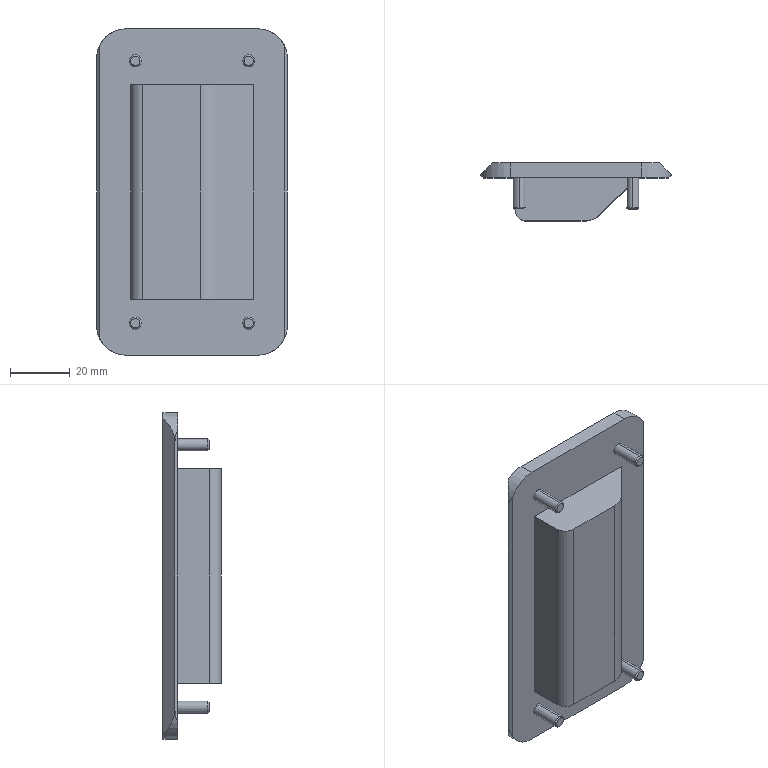Part | SolidWorks | features BaseBody 1 | 1 solid | 49 faces | box 64 x 19.5 x 109.5 mm | volume 34769 mm3 | plane 25 | cylinder 16 | cone 8 | commonest cylinder face diameters 4 x8 20 x4 16 x2 6 x1 8 x1
STEP:
#1=CARTESIAN_POINT('',(19.,-10.5,-45.571));
#2=VERTEX_POINT('',#1);
#3=CARTESIAN_POINT('',(19.,-10.5,-42.429));
#4=VERTEX_POINT('',#3);
#5=CARTESIAN_POINT('',(19.,-10.5,-44.));
#6=DIRECTION('',(0.,-1.,0.));
#7=DIRECTION('',(0.,0.,-1.));
#8=AXIS2_PLACEMENT_3D('',#5,#6,#7);
#9=CIRCLE('',#8,1.571);
#10=EDGE_CURVE('',#2,#4,#9,.T.);
#11=ORIENTED_EDGE('',*,*,#10,.F.);
#12=CARTESIAN_POINT('',(19.,-10.07,-46.));
#13=VERTEX_POINT('',#12);
#14=CARTESIAN_POINT('',(19.,-10.07,-46.));
#15=DIRECTION('',(0.,0.7071,-0.7071));
#16=VECTOR('',#15,1000.);
#17=LINE('',#14,#16);
#18=EDGE_CURVE('',#2,#13,#17,.T.);
#19=ORIENTED_EDGE('',*,*,#18,.T.);
#20=CARTESIAN_POINT('',(19.,-10.07,-42.));
#21=VERTEX_POINT('',#20);
#22=CARTESIAN_POINT('',(19.,-10.07,-44.));
#23=DIRECTION('',(0.,-1.,0.));
#24=DIRECTION('',(0.,0.,-1.));
#25=AXIS2_PLACEMENT_3D('',#22,#23,#24);
#26=CIRCLE('',#25,2.);
#27=EDGE_CURVE('',#13,#21,#26,.T.);
#28=ORIENTED_EDGE('',*,*,#27,.T.);
#29=CARTESIAN_POINT('',(19.,-10.07,-42.));
#30=DIRECTION('',(0.,0.7071,0.7071));
#31=VECTOR('',#30,1000.);
#32=LINE('',#29,#31);
#33=EDGE_CURVE('',#4,#21,#32,.T.);
#34=ORIENTED_EDGE('',*,*,#33,.F.);
#35=EDGE_LOOP('',(#11,#19,#28,#34));
#36=FACE_OUTER_BOUND('',#35,.T.);
#37=CARTESIAN_POINT('',(19.,-10.07,-44.));
#38=DIRECTION('',(0.,1.,0.));
#39=DIRECTION('',(0.,0.,1.));
#40=AXIS2_PLACEMENT_3D('',#37,#38,#39);
#41=CONICAL_SURFACE('',#40,2.,0.7854);
#42=ADVANCED_FACE('',(#36),#41,.T.);
#43=CARTESIAN_POINT('',(19.,0.,-46.));
#44=VERTEX_POINT('',#43);
#45=CARTESIAN_POINT('',(19.,0.,-42.));
#46=VERTEX_POINT('',#45);
#47=CARTESIAN_POINT('',(19.,0.,-44.));
#48=DIRECTION('',(0.,-1.,0.));
#49=DIRECTION('',(0.,0.,1.));
#50=AXIS2_PLACEMENT_3D('',#47,#48,#49);
#51=CIRCLE('',#50,2.);
#52=EDGE_CURVE('',#44,#46,#51,.T.);
#53=ORIENTED_EDGE('',*,*,#52,.T.);
#54=CARTESIAN_POINT('',(19.,-10.5,-42.));
#55=DIRECTION('',(0.,-1.,0.));
#56=VECTOR('',#55,1000.);
#57=LINE('',#54,#56);
#58=EDGE_CURVE('',#46,#21,#57,.T.);
#59=ORIENTED_EDGE('',*,*,#58,.T.);
#60=ORIENTED_EDGE('',*,*,#27,.F.);
#61=CARTESIAN_POINT('',(19.,-10.5,-46.));
#62=DIRECTION('',(0.,-1.,0.));
#63=VECTOR('',#62,1000.);
#64=LINE('',#61,#63);
#65=EDGE_CURVE('',#44,#13,#64,.T.);
#66=ORIENTED_EDGE('',*,*,#65,.F.);
#67=EDGE_LOOP('',(#53,#59,#60,#66));
#68=FACE_OUTER_BOUND('',#67,.T.);
#69=CARTESIAN_POINT('',(19.,-10.5,-44.));
#70=DIRECTION('',(0.,-1.,0.));
#71=DIRECTION('',(0.,0.,-1.));
#72=AXIS2_PLACEMENT_3D('',#69,#70,#71);
#73=CYLINDRICAL_SURFACE('',#72,2.);
#74=ADVANCED_FACE('',(#68),#73,.T.);
#75=CARTESIAN_POINT('',(-19.,-10.5,-45.571));
#76=VERTEX_POINT('',#75);
#77=CARTESIAN_POINT('',(-19.,-10.5,-42.429));
#78=VERTEX_POINT('',#77);
#79=CARTESIAN_POINT('',(-19.,-10.5,-44.));
#80=DIRECTION('',(0.,-1.,0.));
#81=DIRECTION('',(0.,0.,-1.));
#82=AXIS2_PLACEMENT_3D('',#79,#80,#81);
#83=CIRCLE('',#82,1.571);
#84=EDGE_CURVE('',#76,#78,#83,.T.);
#85=ORIENTED_EDGE('',*,*,#84,.F.);
#86=CARTESIAN_POINT('',(-19.,-10.07,-46.));
#87=VERTEX_POINT('',#86);
#88=CARTESIAN_POINT('',(-19.,-10.07,-46.));
#89=DIRECTION('',(0.,0.7071,-0.7071));
#90=VECTOR('',#89,1000.);
#91=LINE('',#88,#90);
#92=EDGE_CURVE('',#76,#87,#91,.T.);
#93=ORIENTED_EDGE('',*,*,#92,.T.);
#94=CARTESIAN_POINT('',(-19.,-10.07,-42.));
#95=VERTEX_POINT('',#94);
#96=CARTESIAN_POINT('',(-19.,-10.07,-44.));
#97=DIRECTION('',(0.,-1.,0.));
#98=DIRECTION('',(0.,0.,-1.));
#99=AXIS2_PLACEMENT_3D('',#96,#97,#98);
#100=CIRCLE('',#99,2.);
#101=EDGE_CURVE('',#87,#95,#100,.T.);
#102=ORIENTED_EDGE('',*,*,#101,.T.);
#103=CARTESIAN_POINT('',(-19.,-10.07,-42.));
#104=DIRECTION('',(0.,0.7071,0.7071));
#105=VECTOR('',#104,1000.);
#106=LINE('',#103,#105);
#107=EDGE_CURVE('',#78,#95,#106,.T.);
#108=ORIENTED_EDGE('',*,*,#107,.F.);
#109=EDGE_LOOP('',(#85,#93,#102,#108));
#110=FACE_OUTER_BOUND('',#109,.T.);
#111=CARTESIAN_POINT('',(-19.,-10.07,-44.));
#112=DIRECTION('',(0.,1.,0.));
#113=DIRECTION('',(0.,0.,1.));
#114=AXIS2_PLACEMENT_3D('',#111,#112,#113);
#115=CONICAL_SURFACE('',#114,2.,0.7854);
#116=ADVANCED_FACE('',(#110),#115,.T.);
#117=CARTESIAN_POINT('',(-19.,0.,-46.));
#118=VERTEX_POINT('',#117);
#119=CARTESIAN_POINT('',(-19.,0.,-42.));
#120=VERTEX_POINT('',#119);
#121=CARTESIAN_POINT('',(-19.,0.,-44.));
#122=DIRECTION('',(0.,-1.,0.));
#123=DIRECTION('',(0.,0.,1.));
#124=AXIS2_PLACEMENT_3D('',#121,#122,#123);
#125=CIRCLE('',#124,2.);
#126=EDGE_CURVE('',#118,#120,#125,.T.);
#127=ORIENTED_EDGE('',*,*,#126,.T.);
#128=CARTESIAN_POINT('',(-19.,-10.5,-42.));
#129=DIRECTION('',(0.,-1.,0.));
#130=VECTOR('',#129,1000.);
#131=LINE('',#128,#130);
#132=EDGE_CURVE('',#120,#95,#131,.T.);
#133=ORIENTED_EDGE('',*,*,#132,.T.);
#134=ORIENTED_EDGE('',*,*,#101,.F.);
#135=CARTESIAN_POINT('',(-19.,-10.5,-46.));
#136=DIRECTION('',(0.,-1.,0.));
#137=VECTOR('',#136,1000.);
#138=LINE('',#135,#137);
#139=EDGE_CURVE('',#118,#87,#138,.T.);
#140=ORIENTED_EDGE('',*,*,#139,.F.);
#141=EDGE_LOOP('',(#127,#133,#134,#140));
#142=FACE_OUTER_BOUND('',#141,.T.);
#143=CARTESIAN_POINT('',(-19.,-10.5,-44.));
#144=DIRECTION('',(0.,-1.,0.));
#145=DIRECTION('',(0.,0.,-1.));
#146=AXIS2_PLACEMENT_3D('',#143,#144,#145);
#147=CYLINDRICAL_SURFACE('',#146,2.);
#148=ADVANCED_FACE('',(#142),#147,.T.);
#149=CARTESIAN_POINT('',(19.,-10.5,42.429));
#150=VERTEX_POINT('',#149);
#151=CARTESIAN_POINT('',(19.,-10.5,45.571));
#152=VERTEX_POINT('',#151);
#153=CARTESIAN_POINT('',(19.,-10.5,44.));
#154=DIRECTION('',(0.,-1.,0.));
#155=DIRECTION('',(0.,0.,-1.));
#156=AXIS2_PLACEMENT_3D('',#153,#154,#155);
#157=CIRCLE('',#156,1.571);
#158=EDGE_CURVE('',#150,#152,#157,.T.);
#159=ORIENTED_EDGE('',*,*,#158,.F.);
#160=CARTESIAN_POINT('',(19.,-10.07,42.));
#161=VERTEX_POINT('',#160);
#162=CARTESIAN_POINT('',(19.,-10.07,42.));
#163=DIRECTION('',(0.,0.7071,-0.7071));
#164=VECTOR('',#163,1000.);
#165=LINE('',#162,#164);
#166=EDGE_CURVE('',#150,#161,#165,.T.);
#167=ORIENTED_EDGE('',*,*,#166,.T.);
#168=CARTESIAN_POINT('',(19.,-10.07,46.));
#169=VERTEX_POINT('',#168);
#170=CARTESIAN_POINT('',(19.,-10.07,44.));
#171=DIRECTION('',(0.,-1.,0.));
#172=DIRECTION('',(0.,0.,-1.));
#173=AXIS2_PLACEMENT_3D('',#170,#171,#172);
#174=CIRCLE('',#173,2.);
#175=EDGE_CURVE('',#161,#169,#174,.T.);
#176=ORIENTED_EDGE('',*,*,#175,.T.);
#177=CARTESIAN_POINT('',(19.,-10.07,46.));
#178=DIRECTION('',(0.,0.7071,0.7071));
#179=VECTOR('',#178,1000.);
#180=LINE('',#177,#179);
#181=EDGE_CURVE('',#152,#169,#180,.T.);
#182=ORIENTED_EDGE('',*,*,#181,.F.);
#183=EDGE_LOOP('',(#159,#167,#176,#182));
#184=FACE_OUTER_BOUND('',#183,.T.);
#185=CARTESIAN_POINT('',(19.,-10.07,44.));
#186=DIRECTION('',(0.,1.,0.));
#187=DIRECTION('',(0.,0.,1.));
#188=AXIS2_PLACEMENT_3D('',#185,#186,#187);
#189=CONICAL_SURFACE('',#188,2.,0.7854);
#190=ADVANCED_FACE('',(#184),#189,.T.);
#191=CARTESIAN_POINT('',(19.,0.,42.));
#192=VERTEX_POINT('',#191);
#193=CARTESIAN_POINT('',(19.,0.,46.));
#194=VERTEX_POINT('',#193);
#195=CARTESIAN_POINT('',(19.,0.,44.));
#196=DIRECTION('',(0.,-1.,0.));
#197=DIRECTION('',(0.,0.,1.));
#198=AXIS2_PLACEMENT_3D('',#195,#196,#197);
#199=CIRCLE('',#198,2.);
#200=EDGE_CURVE('',#192,#194,#199,.T.);
#201=ORIENTED_EDGE('',*,*,#200,.T.);
#202=CARTESIAN_POINT('',(19.,-10.5,46.));
#203=DIRECTION('',(0.,-1.,0.));
#204=VECTOR('',#203,1000.);
#205=LINE('',#202,#204);
#206=EDGE_CURVE('',#194,#169,#205,.T.);
#207=ORIENTED_EDGE('',*,*,#206,.T.);
#208=ORIENTED_EDGE('',*,*,#175,.F.);
#209=CARTESIAN_POINT('',(19.,-10.5,42.));
#210=DIRECTION('',(0.,-1.,0.));
#211=VECTOR('',#210,1000.);
#212=LINE('',#209,#211);
#213=EDGE_CURVE('',#192,#161,#212,.T.);
#214=ORIENTED_EDGE('',*,*,#213,.F.);
#215=EDGE_LOOP('',(#201,#207,#208,#214));
#216=FACE_OUTER_BOUND('',#215,.T.);
#217=CARTESIAN_POINT('',(19.,-10.5,44.));
#218=DIRECTION('',(0.,-1.,0.));
#219=DIRECTION('',(0.,0.,-1.));
#220=AXIS2_PLACEMENT_3D('',#217,#218,#219);
#221=CYLINDRICAL_SURFACE('',#220,2.);
#222=ADVANCED_FACE('',(#216),#221,.T.);
#223=CARTESIAN_POINT('',(-19.,-10.5,42.429));
#224=VERTEX_POINT('',#223);
#225=CARTESIAN_POINT('',(-19.,-10.5,45.571));
#226=VERTEX_POINT('',#225);
#227=CARTESIAN_POINT('',(-19.,-10.5,44.));
#228=DIRECTION('',(0.,-1.,0.));
#229=DIRECTION('',(0.,0.,-1.));
#230=AXIS2_PLACEMENT_3D('',#227,#228,#229);
#231=CIRCLE('',#230,1.571);
#232=EDGE_CURVE('',#224,#226,#231,.T.);
#233=ORIENTED_EDGE('',*,*,#232,.F.);
#234=CARTESIAN_POINT('',(-19.,-10.07,42.));
#235=VERTEX_POINT('',#234);
#236=CARTESIAN_POINT('',(-19.,-10.07,42.));
#237=DIRECTION('',(0.,0.7071,-0.7071));
#238=VECTOR('',#237,1000.);
#239=LINE('',#236,#238);
#240=EDGE_CURVE('',#224,#235,#239,.T.);
#241=ORIENTED_EDGE('',*,*,#240,.T.);
#242=CARTESIAN_POINT('',(-19.,-10.07,46.));
#243=VERTEX_POINT('',#242);
#244=CARTESIAN_POINT('',(-19.,-10.07,44.));
#245=DIRECTION('',(0.,-1.,0.));
#246=DIRECTION('',(0.,0.,-1.));
#247=AXIS2_PLACEMENT_3D('',#244,#245,#246);
#248=CIRCLE('',#247,2.);
#249=EDGE_CURVE('',#235,#243,#248,.T.);
#250=ORIENTED_EDGE('',*,*,#249,.T.);
#251=CARTESIAN_POINT('',(-19.,-10.07,46.));
#252=DIRECTION('',(0.,0.7071,0.7071));
#253=VECTOR('',#252,1000.);
#254=LINE('',#251,#253);
#255=EDGE_CURVE('',#226,#243,#254,.T.);
#256=ORIENTED_EDGE('',*,*,#255,.F.);
#257=EDGE_LOOP('',(#233,#241,#250,#256));
#258=FACE_OUTER_BOUND('',#257,.T.);
#259=CARTESIAN_POINT('',(-19.,-10.07,44.));
#260=DIRECTION('',(0.,1.,0.));
#261=DIRECTION('',(0.,0.,1.));
#262=AXIS2_PLACEMENT_3D('',#259,#260,#261);
#263=CONICAL_SURFACE('',#262,2.,0.7854);
#264=ADVANCED_FACE('',(#258),#263,.T.);
#265=CARTESIAN_POINT('',(-19.,0.,42.));
#266=VERTEX_POINT('',#265);
#267=CARTESIAN_POINT('',(-19.,0.,46.));
#268=VERTEX_POINT('',#267);
#269=CARTESIAN_POINT('',(-19.,0.,44.));
#270=DIRECTION('',(0.,-1.,0.));
#271=DIRECTION('',(0.,0.,1.));
#272=AXIS2_PLACEMENT_3D('',#269,#270,#271);
#273=CIRCLE('',#272,2.);
#274=EDGE_CURVE('',#266,#268,#273,.T.);
#275=ORIENTED_EDGE('',*,*,#274,.T.);
#276=CARTESIAN_POINT('',(-19.,-10.5,46.));
#277=DIRECTION('',(0.,-1.,0.));
#278=VECTOR('',#277,1000.);
#279=LINE('',#276,#278);
#280=EDGE_CURVE('',#268,#243,#279,.T.);
#281=ORIENTED_EDGE('',*,*,#280,.T.);
#282=ORIENTED_EDGE('',*,*,#249,.F.);
#283=CARTESIAN_POINT('',(-19.,-10.5,42.));
#284=DIRECTION('',(0.,-1.,0.));
#285=VECTOR('',#284,1000.);
#286=LINE('',#283,#285);
#287=EDGE_CURVE('',#266,#235,#286,.T.);
#288=ORIENTED_EDGE('',*,*,#287,.F.);
#289=EDGE_LOOP('',(#275,#281,#282,#288));
#290=FACE_OUTER_BOUND('',#289,.T.);
#291=CARTESIAN_POINT('',(-19.,-10.5,44.));
#292=DIRECTION('',(0.,-1.,0.));
#293=DIRECTION('',(0.,0.,-1.));
#294=AXIS2_PLACEMENT_3D('',#291,#292,#293);
#295=CYLINDRICAL_SURFACE('',#294,2.);
#296=ADVANCED_FACE('',(#290),#295,.T.);
#297=CARTESIAN_POINT('',(19.,-10.5,-44.));
#298=DIRECTION('',(0.,-1.,0.));
#299=DIRECTION('',(0.,0.,-1.));
#300=AXIS2_PLACEMENT_3D('',#297,#298,#299);
#301=CIRCLE('',#300,1.571);
#302=EDGE_CURVE('',#4,#2,#301,.T.);
#303=ORIENTED_EDGE('',*,*,#302,.T.);
#304=ORIENTED_EDGE('',*,*,#10,.T.);
#305=EDGE_LOOP('',(#303,#304));
#306=FACE_OUTER_BOUND('',#305,.T.);
#307=CARTESIAN_POINT('',(20.57,-10.5,-44.));
#308=DIRECTION('',(0.,1.,0.));
#309=DIRECTION('',(1.,0.,0.));
#310=AXIS2_PLACEMENT_3D('',#307,#308,#309);
#311=PLANE('',#310);
#312=ADVANCED_FACE('',(#306),#311,.F.);
#313=CARTESIAN_POINT('',(-19.,-10.5,-44.));
#314=DIRECTION('',(0.,-1.,0.));
#315=DIRECTION('',(0.,0.,-1.));
#316=AXIS2_PLACEMENT_3D('',#313,#314,#315);
#317=CIRCLE('',#316,1.571);
#318=EDGE_CURVE('',#78,#76,#317,.T.);
#319=ORIENTED_EDGE('',*,*,#318,.T.);
#320=ORIENTED_EDGE('',*,*,#84,.T.);
#321=EDGE_LOOP('',(#319,#320));
#322=FACE_OUTER_BOUND('',#321,.T.);
#323=CARTESIAN_POINT('',(-17.43,-10.5,-44.));
#324=DIRECTION('',(0.,1.,0.));
#325=DIRECTION('',(1.,0.,0.));
#326=AXIS2_PLACEMENT_3D('',#323,#324,#325);
#327=PLANE('',#326);
#328=ADVANCED_FACE('',(#322),#327,.F.);
#329=CARTESIAN_POINT('',(19.,-10.5,44.));
#330=DIRECTION('',(0.,-1.,0.));
#331=DIRECTION('',(0.,0.,-1.));
#332=AXIS2_PLACEMENT_3D('',#329,#330,#331);
#333=CIRCLE('',#332,1.571);
#334=EDGE_CURVE('',#152,#150,#333,.T.);
#335=ORIENTED_EDGE('',*,*,#334,.T.);
#336=ORIENTED_EDGE('',*,*,#158,.T.);
#337=EDGE_LOOP('',(#335,#336));
#338=FACE_OUTER_BOUND('',#337,.T.);
#339=CARTESIAN_POINT('',(20.57,-10.5,44.));
#340=DIRECTION('',(0.,1.,0.));
#341=DIRECTION('',(1.,0.,0.));
#342=AXIS2_PLACEMENT_3D('',#339,#340,#341);
#343=PLANE('',#342);
#344=ADVANCED_FACE('',(#338),#343,.F.);
#345=CARTESIAN_POINT('',(-19.,-10.5,44.));
#346=DIRECTION('',(0.,-1.,0.));
#347=DIRECTION('',(0.,0.,-1.));
#348=AXIS2_PLACEMENT_3D('',#345,#346,#347);
#349=CIRCLE('',#348,1.571);
#350=EDGE_CURVE('',#226,#224,#349,.T.);
#351=ORIENTED_EDGE('',*,*,#350,.T.);
#352=ORIENTED_EDGE('',*,*,#232,.T.);
#353=EDGE_LOOP('',(#351,#352));
#354=FACE_OUTER_BOUND('',#353,.T.);
#355=CARTESIAN_POINT('',(-17.43,-10.5,44.));
#356=DIRECTION('',(0.,1.,0.));
#357=DIRECTION('',(1.,0.,0.));
#358=AXIS2_PLACEMENT_3D('',#355,#356,#357);
#359=PLANE('',#358);
#360=ADVANCED_FACE('',(#354),#359,.F.);
#361=CARTESIAN_POINT('',(-18.,2.5,-34.5));
#362=VERTEX_POINT('',#361);
#363=CARTESIAN_POINT('',(-18.,-9.5,-34.5));
#364=VERTEX_POINT('',#363);
#365=CARTESIAN_POINT('',(-18.,2.5,-34.5));
#366=DIRECTION('',(0.,-1.,0.));
#367=VECTOR('',#366,1000.);
#368=LINE('',#365,#367);
#369=EDGE_CURVE('',#362,#364,#368,.T.);
#370=ORIENTED_EDGE('',*,*,#369,.T.);
#371=CARTESIAN_POINT('',(-15.,-12.5,-34.5));
#372=VERTEX_POINT('',#371);
#373=CARTESIAN_POINT('',(-15.,-9.5,-34.5));
#374=DIRECTION('',(0.,0.,1.));
#375=DIRECTION('',(1.,0.,0.));
#376=AXIS2_PLACEMENT_3D('',#373,#374,#375);
#377=CIRCLE('',#376,3.);
#378=EDGE_CURVE('',#364,#372,#377,.T.);
#379=ORIENTED_EDGE('',*,*,#378,.T.);
#380=CARTESIAN_POINT('',(-0.3137,-12.5,-34.5));
#381=VERTEX_POINT('',#380);
#382=CARTESIAN_POINT('',(-15.,-12.5,-34.5));
#383=DIRECTION('',(1.,0.,0.));
#384=VECTOR('',#383,1000.);
#385=LINE('',#382,#384);
#386=EDGE_CURVE('',#372,#381,#385,.T.);
#387=ORIENTED_EDGE('',*,*,#386,.T.);
#388=CARTESIAN_POINT('',(5.343,-10.157,-34.5));
#389=VERTEX_POINT('',#388);
#390=CARTESIAN_POINT('',(-0.3137,-4.5,-34.5));
#391=DIRECTION('',(0.,0.,1.));
#392=DIRECTION('',(1.,0.,0.));
#393=AXIS2_PLACEMENT_3D('',#390,#391,#392);
#394=CIRCLE('',#393,8.);
#395=EDGE_CURVE('',#381,#389,#394,.T.);
#396=ORIENTED_EDGE('',*,*,#395,.T.);
#397=CARTESIAN_POINT('',(18.,2.5,-34.5));
#398=VERTEX_POINT('',#397);
#399=CARTESIAN_POINT('',(5.343,-10.157,-34.5));
#400=DIRECTION('',(0.7071,0.7071,0.));
#401=VECTOR('',#400,1000.);
#402=LINE('',#399,#401);
#403=EDGE_CURVE('',#389,#398,#402,.T.);
#404=ORIENTED_EDGE('',*,*,#403,.T.);
#405=CARTESIAN_POINT('',(18.,5.,-34.5));
#406=VERTEX_POINT('',#405);
#407=CARTESIAN_POINT('',(18.,2.5,-34.5));
#408=DIRECTION('',(0.,1.,0.));
#409=VECTOR('',#408,1000.);
#410=LINE('',#407,#409);
#411=EDGE_CURVE('',#398,#406,#410,.T.);
#412=ORIENTED_EDGE('',*,*,#411,.T.);
#413=CARTESIAN_POINT('',(-7.,5.,-34.5));
#414=VERTEX_POINT('',#413);
#415=CARTESIAN_POINT('',(18.,5.,-34.5));
#416=DIRECTION('',(-1.,0.,0.));
#417=VECTOR('',#416,1000.);
#418=LINE('',#415,#417);
#419=EDGE_CURVE('',#406,#414,#418,.T.);
#420=ORIENTED_EDGE('',*,*,#419,.T.);
#421=CARTESIAN_POINT('',(-7.,2.5,-34.5));
#422=VERTEX_POINT('',#421);
#423=CARTESIAN_POINT('',(-7.,5.,-34.5));
#424=DIRECTION('',(0.,-1.,0.));
#425=VECTOR('',#424,1000.);
#426=LINE('',#423,#425);
#427=EDGE_CURVE('',#414,#422,#426,.T.);
#428=ORIENTED_EDGE('',*,*,#427,.T.);
#429=CARTESIAN_POINT('',(-7.,2.5,-34.5));
#430=DIRECTION('',(-1.,0.,0.));
#431=VECTOR('',#430,1000.);
#432=LINE('',#429,#431);
#433=EDGE_CURVE('',#422,#362,#432,.T.);
#434=ORIENTED_EDGE('',*,*,#433,.T.);
#435=EDGE_LOOP('',(#370,#379,#387,#396,#404,#412,#420,#428,#434));
#436=FACE_OUTER_BOUND('',#435,.T.);
#437=CARTESIAN_POINT('',(-15.,-9.5,-34.5));
#438=DIRECTION('',(0.,0.,1.));
#439=DIRECTION('',(1.,0.,0.));
#440=AXIS2_PLACEMENT_3D('',#437,#438,#439);
#441=PLANE('',#440);
#442=ADVANCED_FACE('',(#436),#441,.T.);
#443=CARTESIAN_POINT('',(-18.,2.5,34.5));
#444=VERTEX_POINT('',#443);
#445=CARTESIAN_POINT('',(-18.,-9.5,34.5));
#446=VERTEX_POINT('',#445);
#447=CARTESIAN_POINT('',(-18.,2.5,34.5));
#448=DIRECTION('',(0.,-1.,0.));
#449=VECTOR('',#448,1000.);
#450=LINE('',#447,#449);
#451=EDGE_CURVE('',#444,#446,#450,.T.);
#452=ORIENTED_EDGE('',*,*,#451,.F.);
#453=CARTESIAN_POINT('',(-7.,2.5,34.5));
#454=VERTEX_POINT('',#453);
#455=CARTESIAN_POINT('',(-7.,2.5,34.5));
#456=DIRECTION('',(-1.,0.,0.));
#457=VECTOR('',#456,1000.);
#458=LINE('',#455,#457);
#459=EDGE_CURVE('',#454,#444,#458,.T.);
#460=ORIENTED_EDGE('',*,*,#459,.F.);
#461=CARTESIAN_POINT('',(-7.,5.,34.5));
#462=VERTEX_POINT('',#461);
#463=CARTESIAN_POINT('',(-7.,5.,34.5));
#464=DIRECTION('',(0.,-1.,0.));
#465=VECTOR('',#464,1000.);
#466=LINE('',#463,#465);
#467=EDGE_CURVE('',#462,#454,#466,.T.);
#468=ORIENTED_EDGE('',*,*,#467,.F.);
#469=CARTESIAN_POINT('',(18.,5.,34.5));
#470=VERTEX_POINT('',#469);
#471=CARTESIAN_POINT('',(18.,5.,34.5));
#472=DIRECTION('',(-1.,0.,0.));
#473=VECTOR('',#472,1000.);
#474=LINE('',#471,#473);
#475=EDGE_CURVE('',#470,#462,#474,.T.);
#476=ORIENTED_EDGE('',*,*,#475,.F.);
#477=CARTESIAN_POINT('',(18.,2.5,34.5));
#478=VERTEX_POINT('',#477);
#479=CARTESIAN_POINT('',(18.,2.5,34.5));
#480=DIRECTION('',(0.,1.,0.));
#481=VECTOR('',#480,1000.);
#482=LINE('',#479,#481);
#483=EDGE_CURVE('',#478,#470,#482,.T.);
#484=ORIENTED_EDGE('',*,*,#483,.F.);
#485=CARTESIAN_POINT('',(5.343,-10.157,34.5));
#486=VERTEX_POINT('',#485);
#487=CARTESIAN_POINT('',(5.343,-10.157,34.5));
#488=DIRECTION('',(0.7071,0.7071,0.));
#489=VECTOR('',#488,1000.);
#490=LINE('',#487,#489);
#491=EDGE_CURVE('',#486,#478,#490,.T.);
#492=ORIENTED_EDGE('',*,*,#491,.F.);
#493=CARTESIAN_POINT('',(-0.3137,-12.5,34.5));
#494=VERTEX_POINT('',#493);
#495=CARTESIAN_POINT('',(-0.3137,-4.5,34.5));
#496=DIRECTION('',(0.,0.,1.));
#497=DIRECTION('',(1.,0.,0.));
#498=AXIS2_PLACEMENT_3D('',#495,#496,#497);
#499=CIRCLE('',#498,8.);
#500=EDGE_CURVE('',#494,#486,#499,.T.);
#501=ORIENTED_EDGE('',*,*,#500,.F.);
#502=CARTESIAN_POINT('',(-15.,-12.5,34.5));
#503=VERTEX_POINT('',#502);
#504=CARTESIAN_POINT('',(-15.,-12.5,34.5));
#505=DIRECTION('',(1.,0.,0.));
#506=VECTOR('',#505,1000.);
#507=LINE('',#504,#506);
#508=EDGE_CURVE('',#503,#494,#507,.T.);
#509=ORIENTED_EDGE('',*,*,#508,.F.);
#510=CARTESIAN_POINT('',(-15.,-9.5,34.5));
#511=DIRECTION('',(0.,0.,1.));
#512=DIRECTION('',(1.,0.,0.));
#513=AXIS2_PLACEMENT_3D('',#510,#511,#512);
#514=CIRCLE('',#513,3.);
#515=EDGE_CURVE('',#446,#503,#514,.T.);
#516=ORIENTED_EDGE('',*,*,#515,.F.);
#517=EDGE_LOOP('',(#452,#460,#468,#476,#484,#492,#501,#509,#516));
#518=FACE_OUTER_BOUND('',#517,.T.);
#519=CARTESIAN_POINT('',(-15.,-9.5,34.5));
#520=DIRECTION('',(0.,0.,1.));
#521=DIRECTION('',(1.,0.,0.));
#522=AXIS2_PLACEMENT_3D('',#519,#520,#521);
#523=PLANE('',#522);
#524=ADVANCED_FACE('',(#518),#523,.F.);
#525=ORIENTED_EDGE('',*,*,#433,.F.);
#526=CARTESIAN_POINT('',(-7.,2.5,34.5));
#527=DIRECTION('',(0.,0.,-1.));
#528=VECTOR('',#527,1000.);
#529=LINE('',#526,#528);
#530=EDGE_CURVE('',#454,#422,#529,.T.);
#531=ORIENTED_EDGE('',*,*,#530,.F.);
#532=ORIENTED_EDGE('',*,*,#459,.T.);
#533=CARTESIAN_POINT('',(-18.,2.5,34.5));
#534=DIRECTION('',(0.,0.,-1.));
#535=VECTOR('',#534,1000.);
#536=LINE('',#533,#535);
#537=EDGE_CURVE('',#444,#362,#536,.T.);
#538=ORIENTED_EDGE('',*,*,#537,.T.);
#539=EDGE_LOOP('',(#525,#531,#532,#538));
#540=FACE_OUTER_BOUND('',#539,.T.);
#541=CARTESIAN_POINT('',(-7.,2.5,34.5));
#542=DIRECTION('',(0.,-1.,0.));
#543=DIRECTION('',(0.,0.,-1.));
#544=AXIS2_PLACEMENT_3D('',#541,#542,#543);
#545=PLANE('',#544);
#546=ADVANCED_FACE('',(#540),#545,.T.);
#547=ORIENTED_EDGE('',*,*,#427,.F.);
#548=CARTESIAN_POINT('',(-7.,5.,34.5));
#549=DIRECTION('',(0.,0.,-1.));
#550=VECTOR('',#549,1000.);
#551=LINE('',#548,#550);
#552=EDGE_CURVE('',#462,#414,#551,.T.);
#553=ORIENTED_EDGE('',*,*,#552,.F.);
#554=ORIENTED_EDGE('',*,*,#467,.T.);
#555=ORIENTED_EDGE('',*,*,#530,.T.);
#556=EDGE_LOOP('',(#547,#553,#554,#555));
#557=FACE_OUTER_BOUND('',#556,.T.);
#558=CARTESIAN_POINT('',(-7.,5.,34.5));
#559=DIRECTION('',(1.,0.,0.));
#560=DIRECTION('',(0.,1.,0.));
#561=AXIS2_PLACEMENT_3D('',#558,#559,#560);
#562=PLANE('',#561);
#563=ADVANCED_FACE('',(#557),#562,.T.);
#564=ORIENTED_EDGE('',*,*,#411,.F.);
#565=CARTESIAN_POINT('',(18.,2.5,34.5));
#566=DIRECTION('',(0.,0.,-1.));
#567=VECTOR('',#566,1000.);
#568=LINE('',#565,#567);
#569=EDGE_CURVE('',#478,#398,#568,.T.);
#570=ORIENTED_EDGE('',*,*,#569,.F.);
#571=ORIENTED_EDGE('',*,*,#483,.T.);
#572=CARTESIAN_POINT('',(18.,5.,34.5));
#573=DIRECTION('',(0.,0.,-1.));
#574=VECTOR('',#573,1000.);
#575=LINE('',#572,#574);
#576=EDGE_CURVE('',#470,#406,#575,.T.);
#577=ORIENTED_EDGE('',*,*,#576,.T.);
#578=EDGE_LOOP('',(#564,#570,#571,#577));
#579=FACE_OUTER_BOUND('',#578,.T.);
#580=CARTESIAN_POINT('',(18.,2.5,34.5));
#581=DIRECTION('',(-1.,0.,0.));
#582=DIRECTION('',(0.,0.,1.));
#583=AXIS2_PLACEMENT_3D('',#580,#581,#582);
#584=PLANE('',#583);
#585=ADVANCED_FACE('',(#579),#584,.T.);
#586=ORIENTED_EDGE('',*,*,#403,.F.);
#587=CARTESIAN_POINT('',(5.343,-10.157,34.5));
#588=DIRECTION('',(0.,0.,-1.));
#589=VECTOR('',#588,1000.);
#590=LINE('',#587,#589);
#591=EDGE_CURVE('',#486,#389,#590,.T.);
#592=ORIENTED_EDGE('',*,*,#591,.F.);
#593=ORIENTED_EDGE('',*,*,#491,.T.);
#594=ORIENTED_EDGE('',*,*,#569,.T.);
#595=EDGE_LOOP('',(#586,#592,#593,#594));
#596=FACE_OUTER_BOUND('',#595,.T.);
#597=CARTESIAN_POINT('',(5.343,-10.157,34.5));
#598=DIRECTION('',(-0.7071,0.7071,0.));
#599=DIRECTION('',(0.,0.,1.));
#600=AXIS2_PLACEMENT_3D('',#597,#598,#599);
#601=PLANE('',#600);
#602=ADVANCED_FACE('',(#596),#601,.T.);
#603=ORIENTED_EDGE('',*,*,#395,.F.);
#604=CARTESIAN_POINT('',(-0.3137,-12.5,34.5));
#605=DIRECTION('',(0.,0.,-1.));
#606=VECTOR('',#605,1000.);
#607=LINE('',#604,#606);
#608=EDGE_CURVE('',#494,#381,#607,.T.);
#609=ORIENTED_EDGE('',*,*,#608,.F.);
#610=ORIENTED_EDGE('',*,*,#500,.T.);
#611=ORIENTED_EDGE('',*,*,#591,.T.);
#612=EDGE_LOOP('',(#603,#609,#610,#611));
#613=FACE_OUTER_BOUND('',#612,.T.);
#614=CARTESIAN_POINT('',(-0.3137,-4.5,34.5));
#615=DIRECTION('',(0.,0.,-1.));
#616=DIRECTION('',(-1.,0.,0.));
#617=AXIS2_PLACEMENT_3D('',#614,#615,#616);
#618=CYLINDRICAL_SURFACE('',#617,8.);
#619=ADVANCED_FACE('',(#613),#618,.F.);
#620=ORIENTED_EDGE('',*,*,#386,.F.);
#621=CARTESIAN_POINT('',(-15.,-12.5,34.5));
#622=DIRECTION('',(0.,0.,-1.));
#623=VECTOR('',#622,1000.);
#624=LINE('',#621,#623);
#625=EDGE_CURVE('',#503,#372,#624,.T.);
#626=ORIENTED_EDGE('',*,*,#625,.F.);
#627=ORIENTED_EDGE('',*,*,#508,.T.);
#628=ORIENTED_EDGE('',*,*,#608,.T.);
#629=EDGE_LOOP('',(#620,#626,#627,#628));
#630=FACE_OUTER_BOUND('',#629,.T.);
#631=CARTESIAN_POINT('',(-15.,-12.5,34.5));
#632=DIRECTION('',(0.,1.,0.));
#633=DIRECTION('',(1.,0.,0.));
#634=AXIS2_PLACEMENT_3D('',#631,#632,#633);
#635=PLANE('',#634);
#636=ADVANCED_FACE('',(#630),#635,.T.);
#637=ORIENTED_EDGE('',*,*,#378,.F.);
#638=CARTESIAN_POINT('',(-18.,-9.5,34.5));
#639=DIRECTION('',(0.,0.,-1.));
#640=VECTOR('',#639,1000.);
#641=LINE('',#638,#640);
#642=EDGE_CURVE('',#446,#364,#641,.T.);
#643=ORIENTED_EDGE('',*,*,#642,.F.);
#644=ORIENTED_EDGE('',*,*,#515,.T.);
#645=ORIENTED_EDGE('',*,*,#625,.T.);
#646=EDGE_LOOP('',(#637,#643,#644,#645));
#647=FACE_OUTER_BOUND('',#646,.T.);
#648=CARTESIAN_POINT('',(-15.,-9.5,34.5));
#649=DIRECTION('',(0.,0.,-1.));
#650=DIRECTION('',(-1.,0.,0.));
#651=AXIS2_PLACEMENT_3D('',#648,#649,#650);
#652=CYLINDRICAL_SURFACE('',#651,3.);
#653=ADVANCED_FACE('',(#647),#652,.F.);
#654=ORIENTED_EDGE('',*,*,#369,.F.);
#655=ORIENTED_EDGE('',*,*,#537,.F.);
#656=ORIENTED_EDGE('',*,*,#451,.T.);
#657=ORIENTED_EDGE('',*,*,#642,.T.);
#658=EDGE_LOOP('',(#654,#655,#656,#657));
#659=FACE_OUTER_BOUND('',#658,.T.);
#660=CARTESIAN_POINT('',(-18.,2.5,34.5));
#661=DIRECTION('',(1.,0.,0.));
#662=DIRECTION('',(0.,1.,0.));
#663=AXIS2_PLACEMENT_3D('',#660,#661,#662);
#664=PLANE('',#663);
#665=ADVANCED_FACE('',(#659),#664,.T.);
#666=CARTESIAN_POINT('',(22.,5.,-54.75));
#667=VERTEX_POINT('',#666);
#668=CARTESIAN_POINT('',(22.,0.,-54.75));
#669=VERTEX_POINT('',#668);
#670=CARTESIAN_POINT('',(22.,54.75,-54.75));
#671=DIRECTION('',(0.,-1.,0.));
#672=VECTOR('',#671,1000.);
#673=LINE('',#670,#672);
#674=EDGE_CURVE('',#667,#669,#673,.T.);
#675=ORIENTED_EDGE('',*,*,#674,.F.);
#676=CARTESIAN_POINT('',(28.,5.,-52.75));
#677=VERTEX_POINT('',#676);
#678=CARTESIAN_POINT('',(22.,5.,-44.75));
#679=DIRECTION('',(0.,1.,0.));
#680=DIRECTION('',(0.,0.,-1.));
#681=AXIS2_PLACEMENT_3D('',#678,#679,#680);
#682=CIRCLE('',#681,10.);
#683=EDGE_CURVE('',#677,#667,#682,.T.);
#684=ORIENTED_EDGE('',*,*,#683,.F.);
#685=CARTESIAN_POINT('',(32.,1.,-44.75));
#686=VERTEX_POINT('',#685);
#687=CARTESIAN_POINT('',(32.,1.,-44.75));
#688=CARTESIAN_POINT('',(32.,1.,-47.957));
#689=CARTESIAN_POINT('',(30.566,2.434,-50.826));
#690=CARTESIAN_POINT('',(28.,5.,-52.75));
#691=(BOUNDED_CURVE()B_SPLINE_CURVE(3,(#687,#688,#689,#690),.UNSPECIFIED.,.F.,.F.)B_SPLINE_CURVE_WITH_KNOTS((4,4),(0.,0.9273),.UNSPECIFIED.)CURVE()GEOMETRIC_REPRESENTATION_ITEM()RATIONAL_B_SPLINE_CURVE((1.,0.9296,0.9296,1.))REPRESENTATION_ITEM(''));
#692=EDGE_CURVE('',#686,#677,#691,.T.);
#693=ORIENTED_EDGE('',*,*,#692,.F.);
#694=CARTESIAN_POINT('',(31.,0.,-49.109));
#695=VERTEX_POINT('',#694);
#696=CARTESIAN_POINT('',(31.,0.,-49.109));
#697=CARTESIAN_POINT('',(31.661,0.6609,-47.744));
#698=CARTESIAN_POINT('',(32.,1.,-46.266));
#699=CARTESIAN_POINT('',(32.,1.,-44.75));
#700=(BOUNDED_CURVE()B_SPLINE_CURVE(3,(#696,#697,#698,#699),.UNSPECIFIED.,.F.,.F.)B_SPLINE_CURVE_WITH_KNOTS((4,4),(2.691,3.142),.UNSPECIFIED.)CURVE()GEOMETRIC_REPRESENTATION_ITEM()RATIONAL_B_SPLINE_CURVE((1.,0.9831,0.9831,1.))REPRESENTATION_ITEM(''));
#701=EDGE_CURVE('',#695,#686,#700,.T.);
#702=ORIENTED_EDGE('',*,*,#701,.F.);
#703=CARTESIAN_POINT('',(22.,0.,-44.75));
#704=DIRECTION('',(0.,-1.,0.));
#705=DIRECTION('',(0.,0.,1.));
#706=AXIS2_PLACEMENT_3D('',#703,#704,#705);
#707=CIRCLE('',#706,10.);
#708=EDGE_CURVE('',#669,#695,#707,.T.);
#709=ORIENTED_EDGE('',*,*,#708,.F.);
#710=EDGE_LOOP('',(#675,#684,#693,#702,#709));
#711=FACE_OUTER_BOUND('',#710,.T.);
#712=CARTESIAN_POINT('',(22.,54.75,-44.75));
#713=DIRECTION('',(0.,-1.,0.));
#714=DIRECTION('',(0.,0.,-1.));
#715=AXIS2_PLACEMENT_3D('',#712,#713,#714);
#716=CYLINDRICAL_SURFACE('',#715,10.);
#717=ADVANCED_FACE('',(#711),#716,.T.);
#718=CARTESIAN_POINT('',(-22.,5.,-54.75));
#719=VERTEX_POINT('',#718);
#720=CARTESIAN_POINT('',(-22.,0.,-54.75));
#721=VERTEX_POINT('',#720);
#722=CARTESIAN_POINT('',(-22.,54.75,-54.75));
#723=DIRECTION('',(0.,-1.,0.));
#724=VECTOR('',#723,1000.);
#725=LINE('',#722,#724);
#726=EDGE_CURVE('',#719,#721,#725,.T.);
#727=ORIENTED_EDGE('',*,*,#726,.F.);
#728=CARTESIAN_POINT('',(28.,5.,-54.75));
#729=DIRECTION('',(-1.,0.,0.));
#730=VECTOR('',#729,1000.);
#731=LINE('',#728,#730);
#732=EDGE_CURVE('',#667,#719,#731,.T.);
#733=ORIENTED_EDGE('',*,*,#732,.F.);
#734=ORIENTED_EDGE('',*,*,#674,.T.);
#735=CARTESIAN_POINT('',(20.5,0.,-54.75));
#736=DIRECTION('',(1.,0.,0.));
#737=VECTOR('',#736,1000.);
#738=LINE('',#735,#737);
#739=EDGE_CURVE('',#721,#669,#738,.T.);
#740=ORIENTED_EDGE('',*,*,#739,.F.);
#741=EDGE_LOOP('',(#727,#733,#734,#740));
#742=FACE_OUTER_BOUND('',#741,.T.);
#743=CARTESIAN_POINT('',(22.,54.75,-54.75));
#744=DIRECTION('',(0.,0.,1.));
#745=DIRECTION('',(1.,0.,0.));
#746=AXIS2_PLACEMENT_3D('',#743,#744,#745);
#747=PLANE('',#746);
#748=ADVANCED_FACE('',(#742),#747,.F.);
#749=CARTESIAN_POINT('',(-32.,1.,-44.75));
#750=VERTEX_POINT('',#749);
#751=CARTESIAN_POINT('',(-31.,0.,-49.109));
#752=VERTEX_POINT('',#751);
#753=CARTESIAN_POINT('',(-32.,1.,-44.75));
#754=CARTESIAN_POINT('',(-32.,1.,-46.266));
#755=CARTESIAN_POINT('',(-31.661,0.6609,-47.744));
#756=CARTESIAN_POINT('',(-31.,0.,-49.109));
#757=(BOUNDED_CURVE()B_SPLINE_CURVE(3,(#753,#754,#755,#756),.UNSPECIFIED.,.F.,.F.)B_SPLINE_CURVE_WITH_KNOTS((4,4),(3.142,3.593),.UNSPECIFIED.)CURVE()GEOMETRIC_REPRESENTATION_ITEM()RATIONAL_B_SPLINE_CURVE((1.,0.9831,0.9831,1.))REPRESENTATION_ITEM(''));
#758=EDGE_CURVE('',#750,#752,#757,.T.);
#759=ORIENTED_EDGE('',*,*,#758,.F.);
#760=CARTESIAN_POINT('',(-28.,5.,-52.75));
#761=VERTEX_POINT('',#760);
#762=CARTESIAN_POINT('',(-28.,5.,-52.75));
#763=CARTESIAN_POINT('',(-30.566,2.434,-50.826));
#764=CARTESIAN_POINT('',(-32.,1.,-47.957));
#765=CARTESIAN_POINT('',(-32.,1.,-44.75));
#766=(BOUNDED_CURVE()B_SPLINE_CURVE(3,(#762,#763,#764,#765),.UNSPECIFIED.,.F.,.F.)B_SPLINE_CURVE_WITH_KNOTS((4,4),(5.356,6.283),.UNSPECIFIED.)CURVE()GEOMETRIC_REPRESENTATION_ITEM()RATIONAL_B_SPLINE_CURVE((1.,0.9296,0.9296,1.))REPRESENTATION_ITEM(''));
#767=EDGE_CURVE('',#761,#750,#766,.T.);
#768=ORIENTED_EDGE('',*,*,#767,.F.);
#769=CARTESIAN_POINT('',(-22.,5.,-44.75));
#770=DIRECTION('',(0.,1.,0.));
#771=DIRECTION('',(0.,0.,-1.));
#772=AXIS2_PLACEMENT_3D('',#769,#770,#771);
#773=CIRCLE('',#772,10.);
#774=EDGE_CURVE('',#719,#761,#773,.T.);
#775=ORIENTED_EDGE('',*,*,#774,.F.);
#776=ORIENTED_EDGE('',*,*,#726,.T.);
#777=CARTESIAN_POINT('',(-22.,0.,-44.75));
#778=DIRECTION('',(0.,-1.,0.));
#779=DIRECTION('',(0.,0.,1.));
#780=AXIS2_PLACEMENT_3D('',#777,#778,#779);
#781=CIRCLE('',#780,10.);
#782=EDGE_CURVE('',#752,#721,#781,.T.);
#783=ORIENTED_EDGE('',*,*,#782,.F.);
#784=EDGE_LOOP('',(#759,#768,#775,#776,#783));
#785=FACE_OUTER_BOUND('',#784,.T.);
#786=CARTESIAN_POINT('',(-22.,54.75,-44.75));
#787=DIRECTION('',(0.,-1.,0.));
#788=DIRECTION('',(0.,0.,-1.));
#789=AXIS2_PLACEMENT_3D('',#786,#787,#788);
#790=CYLINDRICAL_SURFACE('',#789,10.);
#791=ADVANCED_FACE('',(#785),#790,.T.);
#792=CARTESIAN_POINT('',(32.,1.,44.75));
#793=VERTEX_POINT('',#792);
#794=CARTESIAN_POINT('',(31.,0.,49.109));
#795=VERTEX_POINT('',#794);
#796=CARTESIAN_POINT('',(32.,1.,44.75));
#797=CARTESIAN_POINT('',(32.,1.,46.266));
#798=CARTESIAN_POINT('',(31.661,0.6609,47.744));
#799=CARTESIAN_POINT('',(31.,0.,49.109));
#800=(BOUNDED_CURVE()B_SPLINE_CURVE(3,(#796,#797,#798,#799),.UNSPECIFIED.,.F.,.F.)B_SPLINE_CURVE_WITH_KNOTS((4,4),(3.142,3.593),.UNSPECIFIED.)CURVE()GEOMETRIC_REPRESENTATION_ITEM()RATIONAL_B_SPLINE_CURVE((1.,0.9831,0.9831,1.))REPRESENTATION_ITEM(''));
#801=EDGE_CURVE('',#793,#795,#800,.T.);
#802=ORIENTED_EDGE('',*,*,#801,.F.);
#803=CARTESIAN_POINT('',(28.,5.,52.75));
#804=VERTEX_POINT('',#803);
#805=CARTESIAN_POINT('',(28.,5.,52.75));
#806=CARTESIAN_POINT('',(30.566,2.434,50.826));
#807=CARTESIAN_POINT('',(32.,1.,47.957));
#808=CARTESIAN_POINT('',(32.,1.,44.75));
#809=(BOUNDED_CURVE()B_SPLINE_CURVE(3,(#805,#806,#807,#808),.UNSPECIFIED.,.F.,.F.)B_SPLINE_CURVE_WITH_KNOTS((4,4),(5.356,6.283),.UNSPECIFIED.)CURVE()GEOMETRIC_REPRESENTATION_ITEM()RATIONAL_B_SPLINE_CURVE((1.,0.9296,0.9296,1.))REPRESENTATION_ITEM(''));
#810=EDGE_CURVE('',#804,#793,#809,.T.);
#811=ORIENTED_EDGE('',*,*,#810,.F.);
#812=CARTESIAN_POINT('',(22.,5.,54.75));
#813=VERTEX_POINT('',#812);
#814=CARTESIAN_POINT('',(22.,5.,44.75));
#815=DIRECTION('',(0.,1.,0.));
#816=DIRECTION('',(0.,0.,-1.));
#817=AXIS2_PLACEMENT_3D('',#814,#815,#816);
#818=CIRCLE('',#817,10.);
#819=EDGE_CURVE('',#813,#804,#818,.T.);
#820=ORIENTED_EDGE('',*,*,#819,.F.);
#821=CARTESIAN_POINT('',(22.,0.,54.75));
#822=VERTEX_POINT('',#821);
#823=CARTESIAN_POINT('',(22.,54.75,54.75));
#824=DIRECTION('',(0.,-1.,0.));
#825=VECTOR('',#824,1000.);
#826=LINE('',#823,#825);
#827=EDGE_CURVE('',#813,#822,#826,.T.);
#828=ORIENTED_EDGE('',*,*,#827,.T.);
#829=CARTESIAN_POINT('',(22.,0.,44.75));
#830=DIRECTION('',(0.,-1.,0.));
#831=DIRECTION('',(0.,0.,1.));
#832=AXIS2_PLACEMENT_3D('',#829,#830,#831);
#833=CIRCLE('',#832,10.);
#834=EDGE_CURVE('',#795,#822,#833,.T.);
#835=ORIENTED_EDGE('',*,*,#834,.F.);
#836=EDGE_LOOP('',(#802,#811,#820,#828,#835));
#837=FACE_OUTER_BOUND('',#836,.T.);
#838=CARTESIAN_POINT('',(22.,54.75,44.75));
#839=DIRECTION('',(0.,-1.,0.));
#840=DIRECTION('',(0.,0.,-1.));
#841=AXIS2_PLACEMENT_3D('',#838,#839,#840);
#842=CYLINDRICAL_SURFACE('',#841,10.);
#843=ADVANCED_FACE('',(#837),#842,.T.);
#844=ORIENTED_EDGE('',*,*,#827,.F.);
#845=CARTESIAN_POINT('',(-22.,5.,54.75));
#846=VERTEX_POINT('',#845);
#847=CARTESIAN_POINT('',(28.,5.,54.75));
#848=DIRECTION('',(1.,0.,0.));
#849=VECTOR('',#848,1000.);
#850=LINE('',#847,#849);
#851=EDGE_CURVE('',#846,#813,#850,.T.);
#852=ORIENTED_EDGE('',*,*,#851,.F.);
#853=CARTESIAN_POINT('',(-22.,0.,54.75));
#854=VERTEX_POINT('',#853);
#855=CARTESIAN_POINT('',(-22.,54.75,54.75));
#856=DIRECTION('',(0.,-1.,0.));
#857=VECTOR('',#856,1000.);
#858=LINE('',#855,#857);
#859=EDGE_CURVE('',#846,#854,#858,.T.);
#860=ORIENTED_EDGE('',*,*,#859,.T.);
#861=CARTESIAN_POINT('',(20.5,0.,54.75));
#862=DIRECTION('',(-1.,0.,0.));
#863=VECTOR('',#862,1000.);
#864=LINE('',#861,#863);
#865=EDGE_CURVE('',#822,#854,#864,.T.);
#866=ORIENTED_EDGE('',*,*,#865,.F.);
#867=EDGE_LOOP('',(#844,#852,#860,#866));
#868=FACE_OUTER_BOUND('',#867,.T.);
#869=CARTESIAN_POINT('',(-22.,54.75,54.75));
#870=DIRECTION('',(0.,0.,-1.));
#871=DIRECTION('',(0.,-1.,0.));
#872=AXIS2_PLACEMENT_3D('',#869,#870,#871);
#873=PLANE('',#872);
#874=ADVANCED_FACE('',(#868),#873,.F.);
#875=ORIENTED_EDGE('',*,*,#859,.F.);
#876=CARTESIAN_POINT('',(-28.,5.,52.75));
#877=VERTEX_POINT('',#876);
#878=CARTESIAN_POINT('',(-22.,5.,44.75));
#879=DIRECTION('',(0.,1.,0.));
#880=DIRECTION('',(0.,0.,-1.));
#881=AXIS2_PLACEMENT_3D('',#878,#879,#880);
#882=CIRCLE('',#881,10.);
#883=EDGE_CURVE('',#877,#846,#882,.T.);
#884=ORIENTED_EDGE('',*,*,#883,.F.);
#885=CARTESIAN_POINT('',(-32.,1.,44.75));
#886=VERTEX_POINT('',#885);
#887=CARTESIAN_POINT('',(-32.,1.,44.75));
#888=CARTESIAN_POINT('',(-32.,1.,47.957));
#889=CARTESIAN_POINT('',(-30.566,2.434,50.826));
#890=CARTESIAN_POINT('',(-28.,5.,52.75));
#891=(BOUNDED_CURVE()B_SPLINE_CURVE(3,(#887,#888,#889,#890),.UNSPECIFIED.,.F.,.F.)B_SPLINE_CURVE_WITH_KNOTS((4,4),(0.,0.9273),.UNSPECIFIED.)CURVE()GEOMETRIC_REPRESENTATION_ITEM()RATIONAL_B_SPLINE_CURVE((1.,0.9296,0.9296,1.))REPRESENTATION_ITEM(''));
#892=EDGE_CURVE('',#886,#877,#891,.T.);
#893=ORIENTED_EDGE('',*,*,#892,.F.);
#894=CARTESIAN_POINT('',(-31.,0.,49.109));
#895=VERTEX_POINT('',#894);
#896=CARTESIAN_POINT('',(-31.,0.,49.109));
#897=CARTESIAN_POINT('',(-31.661,0.6609,47.744));
#898=CARTESIAN_POINT('',(-32.,1.,46.266));
#899=CARTESIAN_POINT('',(-32.,1.,44.75));
#900=(BOUNDED_CURVE()B_SPLINE_CURVE(3,(#896,#897,#898,#899),.UNSPECIFIED.,.F.,.F.)B_SPLINE_CURVE_WITH_KNOTS((4,4),(2.691,3.142),.UNSPECIFIED.)CURVE()GEOMETRIC_REPRESENTATION_ITEM()RATIONAL_B_SPLINE_CURVE((1.,0.9831,0.9831,1.))REPRESENTATION_ITEM(''));
#901=EDGE_CURVE('',#895,#886,#900,.T.);
#902=ORIENTED_EDGE('',*,*,#901,.F.);
#903=CARTESIAN_POINT('',(-22.,0.,44.75));
#904=DIRECTION('',(0.,-1.,0.));
#905=DIRECTION('',(0.,0.,1.));
#906=AXIS2_PLACEMENT_3D('',#903,#904,#905);
#907=CIRCLE('',#906,10.);
#908=EDGE_CURVE('',#854,#895,#907,.T.);
#909=ORIENTED_EDGE('',*,*,#908,.F.);
#910=EDGE_LOOP('',(#875,#884,#893,#902,#909));
#911=FACE_OUTER_BOUND('',#910,.T.);
#912=CARTESIAN_POINT('',(-22.,54.75,44.75));
#913=DIRECTION('',(0.,-1.,0.));
#914=DIRECTION('',(0.,0.,-1.));
#915=AXIS2_PLACEMENT_3D('',#912,#913,#914);
#916=CYLINDRICAL_SURFACE('',#915,10.);
#917=ADVANCED_FACE('',(#911),#916,.T.);
#918=CARTESIAN_POINT('',(8.343,-12.157,-36.));
#919=VERTEX_POINT('',#918);
#920=CARTESIAN_POINT('',(20.5,0.,-36.));
#921=VERTEX_POINT('',#920);
#922=CARTESIAN_POINT('',(8.343,-12.157,-36.));
#923=DIRECTION('',(0.7071,0.7071,0.));
#924=VECTOR('',#923,1000.);
#925=LINE('',#922,#924);
#926=EDGE_CURVE('',#919,#921,#925,.T.);
#927=ORIENTED_EDGE('',*,*,#926,.T.);
#928=CARTESIAN_POINT('',(20.5,0.,36.));
#929=VERTEX_POINT('',#928);
#930=CARTESIAN_POINT('',(20.5,0.,36.));
#931=DIRECTION('',(0.,0.,-1.));
#932=VECTOR('',#931,1000.);
#933=LINE('',#930,#932);
#934=EDGE_CURVE('',#929,#921,#933,.T.);
#935=ORIENTED_EDGE('',*,*,#934,.F.);
#936=CARTESIAN_POINT('',(8.343,-12.157,36.));
#937=VERTEX_POINT('',#936);
#938=CARTESIAN_POINT('',(8.343,-12.157,36.));
#939=DIRECTION('',(0.7071,0.7071,0.));
#940=VECTOR('',#939,1000.);
#941=LINE('',#938,#940);
#942=EDGE_CURVE('',#937,#929,#941,.T.);
#943=ORIENTED_EDGE('',*,*,#942,.F.);
#944=CARTESIAN_POINT('',(8.343,-12.157,36.));
#945=DIRECTION('',(0.,0.,-1.));
#946=VECTOR('',#945,1000.);
#947=LINE('',#944,#946);
#948=EDGE_CURVE('',#937,#919,#947,.T.);
#949=ORIENTED_EDGE('',*,*,#948,.T.);
#950=EDGE_LOOP('',(#927,#935,#943,#949));
#951=FACE_OUTER_BOUND('',#950,.T.);
#952=CARTESIAN_POINT('',(8.343,-12.157,36.));
#953=DIRECTION('',(-0.7071,0.7071,0.));
#954=DIRECTION('',(0.,0.,1.));
#955=AXIS2_PLACEMENT_3D('',#952,#953,#954);
#956=PLANE('',#955);
#957=ADVANCED_FACE('',(#951),#956,.F.);
#958=CARTESIAN_POINT('',(2.686,-14.5,-36.));
#959=VERTEX_POINT('',#958);
#960=CARTESIAN_POINT('',(2.686,-6.5,-36.));
#961=DIRECTION('',(0.,0.,1.));
#962=DIRECTION('',(1.,0.,0.));
#963=AXIS2_PLACEMENT_3D('',#960,#961,#962);
#964=CIRCLE('',#963,8.);
#965=EDGE_CURVE('',#959,#919,#964,.T.);
#966=ORIENTED_EDGE('',*,*,#965,.T.);
#967=ORIENTED_EDGE('',*,*,#948,.F.);
#968=CARTESIAN_POINT('',(2.686,-14.5,36.));
#969=VERTEX_POINT('',#968);
#970=CARTESIAN_POINT('',(2.686,-6.5,36.));
#971=DIRECTION('',(0.,0.,1.));
#972=DIRECTION('',(1.,0.,0.));
#973=AXIS2_PLACEMENT_3D('',#970,#971,#972);
#974=CIRCLE('',#973,8.);
#975=EDGE_CURVE('',#969,#937,#974,.T.);
#976=ORIENTED_EDGE('',*,*,#975,.F.);
#977=CARTESIAN_POINT('',(2.686,-14.5,36.));
#978=DIRECTION('',(0.,0.,-1.));
#979=VECTOR('',#978,1000.);
#980=LINE('',#977,#979);
#981=EDGE_CURVE('',#969,#959,#980,.T.);
#982=ORIENTED_EDGE('',*,*,#981,.T.);
#983=EDGE_LOOP('',(#966,#967,#976,#982));
#984=FACE_OUTER_BOUND('',#983,.T.);
#985=CARTESIAN_POINT('',(2.686,-6.5,36.));
#986=DIRECTION('',(0.,0.,-1.));
#987=DIRECTION('',(-1.,0.,0.));
#988=AXIS2_PLACEMENT_3D('',#985,#986,#987);
#989=CYLINDRICAL_SURFACE('',#988,8.);
#990=ADVANCED_FACE('',(#984),#989,.T.);
#991=CARTESIAN_POINT('',(-16.5,-14.5,-36.));
#992=VERTEX_POINT('',#991);
#993=CARTESIAN_POINT('',(-16.5,-14.5,-36.));
#994=DIRECTION('',(1.,0.,0.));
#995=VECTOR('',#994,1000.);
#996=LINE('',#993,#995);
#997=EDGE_CURVE('',#992,#959,#996,.T.);
#998=ORIENTED_EDGE('',*,*,#997,.T.);
#999=ORIENTED_EDGE('',*,*,#981,.F.);
#1000=CARTESIAN_POINT('',(-16.5,-14.5,36.));
#1001=VERTEX_POINT('',#1000);
#1002=CARTESIAN_POINT('',(-16.5,-14.5,36.));
#1003=DIRECTION('',(1.,0.,0.));
#1004=VECTOR('',#1003,1000.);
#1005=LINE('',#1002,#1004);
#1006=EDGE_CURVE('',#1001,#969,#1005,.T.);
#1007=ORIENTED_EDGE('',*,*,#1006,.F.);
#1008=CARTESIAN_POINT('',(-16.5,-14.5,36.));
#1009=DIRECTION('',(0.,0.,-1.));
#1010=VECTOR('',#1009,1000.);
#1011=LINE('',#1008,#1010);
#1012=EDGE_CURVE('',#1001,#992,#1011,.T.);
#1013=ORIENTED_EDGE('',*,*,#1012,.T.);
#1014=EDGE_LOOP('',(#998,#999,#1007,#1013));
#1015=FACE_OUTER_BOUND('',#1014,.T.);
#1016=CARTESIAN_POINT('',(-16.5,-14.5,36.));
#1017=DIRECTION('',(0.,1.,0.));
#1018=DIRECTION('',(1.,0.,0.));
#1019=AXIS2_PLACEMENT_3D('',#1016,#1017,#1018);
#1020=PLANE('',#1019);
#1021=ADVANCED_FACE('',(#1015),#1020,.F.);
#1022=CARTESIAN_POINT('',(-20.5,-10.5,-36.));
#1023=VERTEX_POINT('',#1022);
#1024=CARTESIAN_POINT('',(-16.5,-10.5,-36.));
#1025=DIRECTION('',(0.,0.,1.));
#1026=DIRECTION('',(1.,0.,0.));
#1027=AXIS2_PLACEMENT_3D('',#1024,#1025,#1026);
#1028=CIRCLE('',#1027,4.);
#1029=EDGE_CURVE('',#1023,#992,#1028,.T.);
#1030=ORIENTED_EDGE('',*,*,#1029,.T.);
#1031=ORIENTED_EDGE('',*,*,#1012,.F.);
#1032=CARTESIAN_POINT('',(-20.5,-10.5,36.));
#1033=VERTEX_POINT('',#1032);
#1034=CARTESIAN_POINT('',(-16.5,-10.5,36.));
#1035=DIRECTION('',(0.,0.,1.));
#1036=DIRECTION('',(1.,0.,0.));
#1037=AXIS2_PLACEMENT_3D('',#1034,#1035,#1036);
#1038=CIRCLE('',#1037,4.);
#1039=EDGE_CURVE('',#1033,#1001,#1038,.T.);
#1040=ORIENTED_EDGE('',*,*,#1039,.F.);
#1041=CARTESIAN_POINT('',(-20.5,-10.5,36.));
#1042=DIRECTION('',(0.,0.,-1.));
#1043=VECTOR('',#1042,1000.);
#1044=LINE('',#1041,#1043);
#1045=EDGE_CURVE('',#1033,#1023,#1044,.T.);
#1046=ORIENTED_EDGE('',*,*,#1045,.T.);
#1047=EDGE_LOOP('',(#1030,#1031,#1040,#1046));
#1048=FACE_OUTER_BOUND('',#1047,.T.);
#1049=CARTESIAN_POINT('',(-16.5,-10.5,36.));
#1050=DIRECTION('',(0.,0.,-1.));
#1051=DIRECTION('',(-1.,0.,0.));
#1052=AXIS2_PLACEMENT_3D('',#1049,#1050,#1051);
#1053=CYLINDRICAL_SURFACE('',#1052,4.);
#1054=ADVANCED_FACE('',(#1048),#1053,.T.);
#1055=CARTESIAN_POINT('',(-20.5,0.,-36.));
#1056=VERTEX_POINT('',#1055);
#1057=CARTESIAN_POINT('',(-20.5,0.,-36.));
#1058=DIRECTION('',(0.,-1.,0.));
#1059=VECTOR('',#1058,1000.);
#1060=LINE('',#1057,#1059);
#1061=EDGE_CURVE('',#1056,#1023,#1060,.T.);
#1062=ORIENTED_EDGE('',*,*,#1061,.T.);
#1063=ORIENTED_EDGE('',*,*,#1045,.F.);
#1064=CARTESIAN_POINT('',(-20.5,0.,36.));
#1065=VERTEX_POINT('',#1064);
#1066=CARTESIAN_POINT('',(-20.5,0.,36.));
#1067=DIRECTION('',(0.,-1.,0.));
#1068=VECTOR('',#1067,1000.);
#1069=LINE('',#1066,#1068);
#1070=EDGE_CURVE('',#1065,#1033,#1069,.T.);
#1071=ORIENTED_EDGE('',*,*,#1070,.F.);
#1072=CARTESIAN_POINT('',(-20.5,0.,36.));
#1073=DIRECTION('',(0.,0.,-1.));
#1074=VECTOR('',#1073,1000.);
#1075=LINE('',#1072,#1074);
#1076=EDGE_CURVE('',#1065,#1056,#1075,.T.);
#1077=ORIENTED_EDGE('',*,*,#1076,.T.);
#1078=EDGE_LOOP('',(#1062,#1063,#1071,#1077));
#1079=FACE_OUTER_BOUND('',#1078,.T.);
#1080=CARTESIAN_POINT('',(-20.5,0.,36.));
#1081=DIRECTION('',(1.,0.,0.));
#1082=DIRECTION('',(0.,1.,0.));
#1083=AXIS2_PLACEMENT_3D('',#1080,#1081,#1082);
#1084=PLANE('',#1083);
#1085=ADVANCED_FACE('',(#1079),#1084,.F.);
#1086=CARTESIAN_POINT('',(-32.,1.,36.));
#1087=DIRECTION('',(0.,0.,-1.));
#1088=VECTOR('',#1087,1000.);
#1089=LINE('',#1086,#1088);
#1090=EDGE_CURVE('',#886,#750,#1089,.T.);
#1091=ORIENTED_EDGE('',*,*,#1090,.T.);
#1092=ORIENTED_EDGE('',*,*,#758,.T.);
#1093=CARTESIAN_POINT('',(-31.,0.,36.));
#1094=DIRECTION('',(0.,0.,-1.));
#1095=VECTOR('',#1094,1000.);
#1096=LINE('',#1093,#1095);
#1097=EDGE_CURVE('',#895,#752,#1096,.T.);
#1098=ORIENTED_EDGE('',*,*,#1097,.F.);
#1099=ORIENTED_EDGE('',*,*,#901,.T.);
#1100=EDGE_LOOP('',(#1091,#1092,#1098,#1099));
#1101=FACE_OUTER_BOUND('',#1100,.T.);
#1102=CARTESIAN_POINT('',(-32.,1.,36.));
#1103=DIRECTION('',(0.7071,0.7071,0.));
#1104=DIRECTION('',(0.,0.,-1.));
#1105=AXIS2_PLACEMENT_3D('',#1102,#1103,#1104);
#1106=PLANE('',#1105);
#1107=ADVANCED_FACE('',(#1101),#1106,.F.);
#1108=CARTESIAN_POINT('',(-28.,5.,36.));
#1109=DIRECTION('',(0.,0.,-1.));
#1110=VECTOR('',#1109,1000.);
#1111=LINE('',#1108,#1110);
#1112=EDGE_CURVE('',#877,#761,#1111,.T.);
#1113=ORIENTED_EDGE('',*,*,#1112,.T.);
#1114=ORIENTED_EDGE('',*,*,#767,.T.);
#1115=ORIENTED_EDGE('',*,*,#1090,.F.);
#1116=ORIENTED_EDGE('',*,*,#892,.T.);
#1117=EDGE_LOOP('',(#1113,#1114,#1115,#1116));
#1118=FACE_OUTER_BOUND('',#1117,.T.);
#1119=CARTESIAN_POINT('',(-28.,5.,36.));
#1120=DIRECTION('',(0.7071,-0.7071,0.));
#1121=DIRECTION('',(0.,0.,-1.));
#1122=AXIS2_PLACEMENT_3D('',#1119,#1120,#1121);
#1123=PLANE('',#1122);
#1124=ADVANCED_FACE('',(#1118),#1123,.F.);
#1125=CARTESIAN_POINT('',(-16.5,0.,-36.));
#1126=DIRECTION('',(-1.,0.,0.));
#1127=VECTOR('',#1126,1000.);
#1128=LINE('',#1125,#1127);
#1129=EDGE_CURVE('',#921,#1056,#1128,.T.);
#1130=ORIENTED_EDGE('',*,*,#1129,.F.);
#1131=ORIENTED_EDGE('',*,*,#926,.F.);
#1132=ORIENTED_EDGE('',*,*,#965,.F.);
#1133=ORIENTED_EDGE('',*,*,#997,.F.);
#1134=ORIENTED_EDGE('',*,*,#1029,.F.);
#1135=ORIENTED_EDGE('',*,*,#1061,.F.);
#1136=EDGE_LOOP('',(#1130,#1131,#1132,#1133,#1134,#1135));
#1137=FACE_OUTER_BOUND('',#1136,.T.);
#1138=CARTESIAN_POINT('',(-16.5,-10.5,-36.));
#1139=DIRECTION('',(0.,0.,1.));
#1140=DIRECTION('',(1.,0.,0.));
#1141=AXIS2_PLACEMENT_3D('',#1138,#1139,#1140);
#1142=PLANE('',#1141);
#1143=ADVANCED_FACE('',(#1137),#1142,.F.);
#1144=ORIENTED_EDGE('',*,*,#942,.T.);
#1145=CARTESIAN_POINT('',(-16.5,0.,36.));
#1146=DIRECTION('',(-1.,0.,0.));
#1147=VECTOR('',#1146,1000.);
#1148=LINE('',#1145,#1147);
#1149=EDGE_CURVE('',#929,#1065,#1148,.T.);
#1150=ORIENTED_EDGE('',*,*,#1149,.T.);
#1151=ORIENTED_EDGE('',*,*,#1070,.T.);
#1152=ORIENTED_EDGE('',*,*,#1039,.T.);
#1153=ORIENTED_EDGE('',*,*,#1006,.T.);
#1154=ORIENTED_EDGE('',*,*,#975,.T.);
#1155=EDGE_LOOP('',(#1144,#1150,#1151,#1152,#1153,#1154));
#1156=FACE_OUTER_BOUND('',#1155,.T.);
#1157=CARTESIAN_POINT('',(-16.5,-10.5,36.));
#1158=DIRECTION('',(0.,0.,1.));
#1159=DIRECTION('',(1.,0.,0.));
#1160=AXIS2_PLACEMENT_3D('',#1157,#1158,#1159);
#1161=PLANE('',#1160);
#1162=ADVANCED_FACE('',(#1156),#1161,.T.);
#1163=ORIENTED_EDGE('',*,*,#576,.F.);
#1164=ORIENTED_EDGE('',*,*,#475,.T.);
#1165=ORIENTED_EDGE('',*,*,#552,.T.);
#1166=ORIENTED_EDGE('',*,*,#419,.F.);
#1167=EDGE_LOOP('',(#1163,#1164,#1165,#1166));
#1168=FACE_BOUND('',#1167,.T.);
#1169=ORIENTED_EDGE('',*,*,#732,.T.);
#1170=ORIENTED_EDGE('',*,*,#774,.T.);
#1171=ORIENTED_EDGE('',*,*,#1112,.F.);
#1172=ORIENTED_EDGE('',*,*,#883,.T.);
#1173=ORIENTED_EDGE('',*,*,#851,.T.);
#1174=ORIENTED_EDGE('',*,*,#819,.T.);
#1175=CARTESIAN_POINT('',(28.,5.,36.));
#1176=DIRECTION('',(0.,0.,-1.));
#1177=VECTOR('',#1176,1000.);
#1178=LINE('',#1175,#1177);
#1179=EDGE_CURVE('',#804,#677,#1178,.T.);
#1180=ORIENTED_EDGE('',*,*,#1179,.T.);
#1181=ORIENTED_EDGE('',*,*,#683,.T.);
#1182=EDGE_LOOP('',(#1169,#1170,#1171,#1172,#1173,#1174,#1180,#1181));
#1183=FACE_OUTER_BOUND('',#1182,.T.);
#1184=CARTESIAN_POINT('',(28.,5.,36.));
#1185=DIRECTION('',(0.,-1.,0.));
#1186=DIRECTION('',(0.,0.,-1.));
#1187=AXIS2_PLACEMENT_3D('',#1184,#1185,#1186);
#1188=PLANE('',#1187);
#1189=ADVANCED_FACE('',(#1168,#1183),#1188,.F.);
#1190=CARTESIAN_POINT('',(32.,1.,36.));
#1191=DIRECTION('',(0.,0.,-1.));
#1192=VECTOR('',#1191,1000.);
#1193=LINE('',#1190,#1192);
#1194=EDGE_CURVE('',#793,#686,#1193,.T.);
#1195=ORIENTED_EDGE('',*,*,#1194,.T.);
#1196=ORIENTED_EDGE('',*,*,#692,.T.);
#1197=ORIENTED_EDGE('',*,*,#1179,.F.);
#1198=ORIENTED_EDGE('',*,*,#810,.T.);
#1199=EDGE_LOOP('',(#1195,#1196,#1197,#1198));
#1200=FACE_OUTER_BOUND('',#1199,.T.);
#1201=CARTESIAN_POINT('',(32.,1.,36.));
#1202=DIRECTION('',(-0.7071,-0.7071,0.));
#1203=DIRECTION('',(-0.7071,0.7071,0.));
#1204=AXIS2_PLACEMENT_3D('',#1201,#1202,#1203);
#1205=PLANE('',#1204);
#1206=ADVANCED_FACE('',(#1200),#1205,.F.);
#1207=CARTESIAN_POINT('',(31.,0.,36.));
#1208=DIRECTION('',(0.,0.,-1.));
#1209=VECTOR('',#1208,1000.);
#1210=LINE('',#1207,#1209);
#1211=EDGE_CURVE('',#795,#695,#1210,.T.);
#1212=ORIENTED_EDGE('',*,*,#1211,.T.);
#1213=ORIENTED_EDGE('',*,*,#701,.T.);
#1214=ORIENTED_EDGE('',*,*,#1194,.F.);
#1215=ORIENTED_EDGE('',*,*,#801,.T.);
#1216=EDGE_LOOP('',(#1212,#1213,#1214,#1215));
#1217=FACE_OUTER_BOUND('',#1216,.T.);
#1218=CARTESIAN_POINT('',(31.,0.,36.));
#1219=DIRECTION('',(-0.7071,0.7071,0.));
#1220=DIRECTION('',(0.,0.,1.));
#1221=AXIS2_PLACEMENT_3D('',#1218,#1219,#1220);
#1222=PLANE('',#1221);
#1223=ADVANCED_FACE('',(#1217),#1222,.F.);
#1224=ORIENTED_EDGE('',*,*,#934,.T.);
#1225=ORIENTED_EDGE('',*,*,#1129,.T.);
#1226=ORIENTED_EDGE('',*,*,#1076,.F.);
#1227=ORIENTED_EDGE('',*,*,#1149,.F.);
#1228=EDGE_LOOP('',(#1224,#1225,#1226,#1227));
#1229=FACE_BOUND('',#1228,.T.);
#1230=ORIENTED_EDGE('',*,*,#274,.F.);
#1231=CARTESIAN_POINT('',(-19.,0.,44.));
#1232=DIRECTION('',(0.,-1.,0.));
#1233=DIRECTION('',(0.,0.,1.));
#1234=AXIS2_PLACEMENT_3D('',#1231,#1232,#1233);
#1235=CIRCLE('',#1234,2.);
#1236=EDGE_CURVE('',#268,#266,#1235,.T.);
#1237=ORIENTED_EDGE('',*,*,#1236,.F.);
#1238=EDGE_LOOP('',(#1230,#1237));
#1239=FACE_BOUND('',#1238,.T.);
#1240=ORIENTED_EDGE('',*,*,#200,.F.);
#1241=CARTESIAN_POINT('',(19.,0.,44.));
#1242=DIRECTION('',(0.,-1.,0.));
#1243=DIRECTION('',(0.,0.,1.));
#1244=AXIS2_PLACEMENT_3D('',#1241,#1242,#1243);
#1245=CIRCLE('',#1244,2.);
#1246=EDGE_CURVE('',#194,#192,#1245,.T.);
#1247=ORIENTED_EDGE('',*,*,#1246,.F.);
#1248=EDGE_LOOP('',(#1240,#1247));
#1249=FACE_BOUND('',#1248,.T.);
#1250=ORIENTED_EDGE('',*,*,#126,.F.);
#1251=CARTESIAN_POINT('',(-19.,0.,-44.));
#1252=DIRECTION('',(0.,-1.,0.));
#1253=DIRECTION('',(0.,0.,1.));
#1254=AXIS2_PLACEMENT_3D('',#1251,#1252,#1253);
#1255=CIRCLE('',#1254,2.);
#1256=EDGE_CURVE('',#120,#118,#1255,.T.);
#1257=ORIENTED_EDGE('',*,*,#1256,.F.);
#1258=EDGE_LOOP('',(#1250,#1257));
#1259=FACE_BOUND('',#1258,.T.);
#1260=ORIENTED_EDGE('',*,*,#52,.F.);
#1261=CARTESIAN_POINT('',(19.,0.,-44.));
#1262=DIRECTION('',(0.,-1.,0.));
#1263=DIRECTION('',(0.,0.,1.));
#1264=AXIS2_PLACEMENT_3D('',#1261,#1262,#1263);
#1265=CIRCLE('',#1264,2.);
#1266=EDGE_CURVE('',#46,#44,#1265,.T.);
#1267=ORIENTED_EDGE('',*,*,#1266,.F.);
#1268=EDGE_LOOP('',(#1260,#1267));
#1269=FACE_BOUND('',#1268,.T.);
#1270=ORIENTED_EDGE('',*,*,#1097,.T.);
#1271=ORIENTED_EDGE('',*,*,#782,.T.);
#1272=ORIENTED_EDGE('',*,*,#739,.T.);
#1273=ORIENTED_EDGE('',*,*,#708,.T.);
#1274=ORIENTED_EDGE('',*,*,#1211,.F.);
#1275=ORIENTED_EDGE('',*,*,#834,.T.);
#1276=ORIENTED_EDGE('',*,*,#865,.T.);
#1277=ORIENTED_EDGE('',*,*,#908,.T.);
#1278=EDGE_LOOP('',(#1270,#1271,#1272,#1273,#1274,#1275,#1276,#1277));
#1279=FACE_OUTER_BOUND('',#1278,.T.);
#1280=CARTESIAN_POINT('',(20.5,0.,36.));
#1281=DIRECTION('',(0.,1.,0.));
#1282=DIRECTION('',(1.,0.,0.));
#1283=AXIS2_PLACEMENT_3D('',#1280,#1281,#1282);
#1284=PLANE('',#1283);
#1285=ADVANCED_FACE('',(#1229,#1239,#1249,#1259,#1269,#1279),#1284,.F.);
#1286=ORIENTED_EDGE('',*,*,#280,.F.);
#1287=ORIENTED_EDGE('',*,*,#1236,.T.);
#1288=ORIENTED_EDGE('',*,*,#287,.T.);
#1289=CARTESIAN_POINT('',(-19.,-10.07,44.));
#1290=DIRECTION('',(0.,-1.,0.));
#1291=DIRECTION('',(0.,0.,-1.));
#1292=AXIS2_PLACEMENT_3D('',#1289,#1290,#1291);
#1293=CIRCLE('',#1292,2.);
#1294=EDGE_CURVE('',#243,#235,#1293,.T.);
#1295=ORIENTED_EDGE('',*,*,#1294,.F.);
#1296=EDGE_LOOP('',(#1286,#1287,#1288,#1295));
#1297=FACE_OUTER_BOUND('',#1296,.T.);
#1298=CARTESIAN_POINT('',(-19.,-10.5,44.));
#1299=DIRECTION('',(0.,-1.,0.));
#1300=DIRECTION('',(0.,0.,-1.));
#1301=AXIS2_PLACEMENT_3D('',#1298,#1299,#1300);
#1302=CYLINDRICAL_SURFACE('',#1301,2.);
#1303=ADVANCED_FACE('',(#1297),#1302,.T.);
#1304=ORIENTED_EDGE('',*,*,#240,.F.);
#1305=ORIENTED_EDGE('',*,*,#350,.F.);
#1306=ORIENTED_EDGE('',*,*,#255,.T.);
#1307=ORIENTED_EDGE('',*,*,#1294,.T.);
#1308=EDGE_LOOP('',(#1304,#1305,#1306,#1307));
#1309=FACE_OUTER_BOUND('',#1308,.T.);
#1310=CARTESIAN_POINT('',(-19.,-10.07,44.));
#1311=DIRECTION('',(0.,1.,0.));
#1312=DIRECTION('',(0.,0.,1.));
#1313=AXIS2_PLACEMENT_3D('',#1310,#1311,#1312);
#1314=CONICAL_SURFACE('',#1313,2.,0.7854);
#1315=ADVANCED_FACE('',(#1309),#1314,.T.);
#1316=ORIENTED_EDGE('',*,*,#206,.F.);
#1317=ORIENTED_EDGE('',*,*,#1246,.T.);
#1318=ORIENTED_EDGE('',*,*,#213,.T.);
#1319=CARTESIAN_POINT('',(19.,-10.07,44.));
#1320=DIRECTION('',(0.,-1.,0.));
#1321=DIRECTION('',(0.,0.,-1.));
#1322=AXIS2_PLACEMENT_3D('',#1319,#1320,#1321);
#1323=CIRCLE('',#1322,2.);
#1324=EDGE_CURVE('',#169,#161,#1323,.T.);
#1325=ORIENTED_EDGE('',*,*,#1324,.F.);
#1326=EDGE_LOOP('',(#1316,#1317,#1318,#1325));
#1327=FACE_OUTER_BOUND('',#1326,.T.);
#1328=CARTESIAN_POINT('',(19.,-10.5,44.));
#1329=DIRECTION('',(0.,-1.,0.));
#1330=DIRECTION('',(0.,0.,-1.));
#1331=AXIS2_PLACEMENT_3D('',#1328,#1329,#1330);
#1332=CYLINDRICAL_SURFACE('',#1331,2.);
#1333=ADVANCED_FACE('',(#1327),#1332,.T.);
#1334=ORIENTED_EDGE('',*,*,#166,.F.);
#1335=ORIENTED_EDGE('',*,*,#334,.F.);
#1336=ORIENTED_EDGE('',*,*,#181,.T.);
#1337=ORIENTED_EDGE('',*,*,#1324,.T.);
#1338=EDGE_LOOP('',(#1334,#1335,#1336,#1337));
#1339=FACE_OUTER_BOUND('',#1338,.T.);
#1340=CARTESIAN_POINT('',(19.,-10.07,44.));
#1341=DIRECTION('',(0.,1.,0.));
#1342=DIRECTION('',(0.,0.,1.));
#1343=AXIS2_PLACEMENT_3D('',#1340,#1341,#1342);
#1344=CONICAL_SURFACE('',#1343,2.,0.7854);
#1345=ADVANCED_FACE('',(#1339),#1344,.T.);
#1346=ORIENTED_EDGE('',*,*,#132,.F.);
#1347=ORIENTED_EDGE('',*,*,#1256,.T.);
#1348=ORIENTED_EDGE('',*,*,#139,.T.);
#1349=CARTESIAN_POINT('',(-19.,-10.07,-44.));
#1350=DIRECTION('',(0.,-1.,0.));
#1351=DIRECTION('',(0.,0.,-1.));
#1352=AXIS2_PLACEMENT_3D('',#1349,#1350,#1351);
#1353=CIRCLE('',#1352,2.);
#1354=EDGE_CURVE('',#95,#87,#1353,.T.);
#1355=ORIENTED_EDGE('',*,*,#1354,.F.);
#1356=EDGE_LOOP('',(#1346,#1347,#1348,#1355));
#1357=FACE_OUTER_BOUND('',#1356,.T.);
#1358=CARTESIAN_POINT('',(-19.,-10.5,-44.));
#1359=DIRECTION('',(0.,-1.,0.));
#1360=DIRECTION('',(0.,0.,-1.));
#1361=AXIS2_PLACEMENT_3D('',#1358,#1359,#1360);
#1362=CYLINDRICAL_SURFACE('',#1361,2.);
#1363=ADVANCED_FACE('',(#1357),#1362,.T.);
#1364=ORIENTED_EDGE('',*,*,#92,.F.);
#1365=ORIENTED_EDGE('',*,*,#318,.F.);
#1366=ORIENTED_EDGE('',*,*,#107,.T.);
#1367=ORIENTED_EDGE('',*,*,#1354,.T.);
#1368=EDGE_LOOP('',(#1364,#1365,#1366,#1367));
#1369=FACE_OUTER_BOUND('',#1368,.T.);
#1370=CARTESIAN_POINT('',(-19.,-10.07,-44.));
#1371=DIRECTION('',(0.,1.,0.));
#1372=DIRECTION('',(0.,0.,1.));
#1373=AXIS2_PLACEMENT_3D('',#1370,#1371,#1372);
#1374=CONICAL_SURFACE('',#1373,2.,0.7854);
#1375=ADVANCED_FACE('',(#1369),#1374,.T.);
#1376=ORIENTED_EDGE('',*,*,#58,.F.);
#1377=ORIENTED_EDGE('',*,*,#1266,.T.);
#1378=ORIENTED_EDGE('',*,*,#65,.T.);
#1379=CARTESIAN_POINT('',(19.,-10.07,-44.));
#1380=DIRECTION('',(0.,-1.,0.));
#1381=DIRECTION('',(0.,0.,-1.));
#1382=AXIS2_PLACEMENT_3D('',#1379,#1380,#1381);
#1383=CIRCLE('',#1382,2.);
#1384=EDGE_CURVE('',#21,#13,#1383,.T.);
#1385=ORIENTED_EDGE('',*,*,#1384,.F.);
#1386=EDGE_LOOP('',(#1376,#1377,#1378,#1385));
#1387=FACE_OUTER_BOUND('',#1386,.T.);
#1388=CARTESIAN_POINT('',(19.,-10.5,-44.));
#1389=DIRECTION('',(0.,-1.,0.));
#1390=DIRECTION('',(0.,0.,-1.));
#1391=AXIS2_PLACEMENT_3D('',#1388,#1389,#1390);
#1392=CYLINDRICAL_SURFACE('',#1391,2.);
#1393=ADVANCED_FACE('',(#1387),#1392,.T.);
#1394=ORIENTED_EDGE('',*,*,#18,.F.);
#1395=ORIENTED_EDGE('',*,*,#302,.F.);
#1396=ORIENTED_EDGE('',*,*,#33,.T.);
#1397=ORIENTED_EDGE('',*,*,#1384,.T.);
#1398=EDGE_LOOP('',(#1394,#1395,#1396,#1397));
#1399=FACE_OUTER_BOUND('',#1398,.T.);
#1400=CARTESIAN_POINT('',(19.,-10.07,-44.));
#1401=DIRECTION('',(0.,1.,0.));
#1402=DIRECTION('',(0.,0.,1.));
#1403=AXIS2_PLACEMENT_3D('',#1400,#1401,#1402);
#1404=CONICAL_SURFACE('',#1403,2.,0.7854);
#1405=ADVANCED_FACE('',(#1399),#1404,.T.);
#1406=CLOSED_SHELL('',(#42,#74,#116,#148,#190,#222,#264,#296,#312,#328,#344,#360,#442,#524,#546,#563,#585,#602,#619,#636,#653,#665,#717,#748,#791,#843,#874,#917,#957,#990,#1021,#1054,#1085,#1107,#1124,#1143,#1162,#1189,#1206,#1223,#1285,#1303,#1315,#1333,#1345,#1363,#1375,#1393,#1405));
#1407=MANIFOLD_SOLID_BREP('',#1406);
#1408=CARTESIAN_POINT('',(0.,0.,0.));
#1409=DIRECTION('',(0.,0.,1.));
#1410=DIRECTION('',(1.,0.,0.));
#1411=AXIS2_PLACEMENT_3D('',#1408,#1409,#1410);
#1412=(LENGTH_UNIT()NAMED_UNIT(*)SI_UNIT(.MILLI.,.METRE.));
#1413=UNCERTAINTY_MEASURE_WITH_UNIT(LENGTH_MEASURE(0.00001),#1412,'','');
#1414=(NAMED_UNIT(*)PLANE_ANGLE_UNIT()SI_UNIT($,.RADIAN.));
#1415=(NAMED_UNIT(*)SI_UNIT($,.STERADIAN.)SOLID_ANGLE_UNIT());
#1416=(GEOMETRIC_REPRESENTATION_CONTEXT(3)GLOBAL_UNCERTAINTY_ASSIGNED_CONTEXT((#1413))GLOBAL_UNIT_ASSIGNED_CONTEXT((#1412,#1414,#1415))REPRESENTATION_CONTEXT('',''));
#1417=ADVANCED_BREP_SHAPE_REPRESENTATION('',(#1407,#1411),#1416);